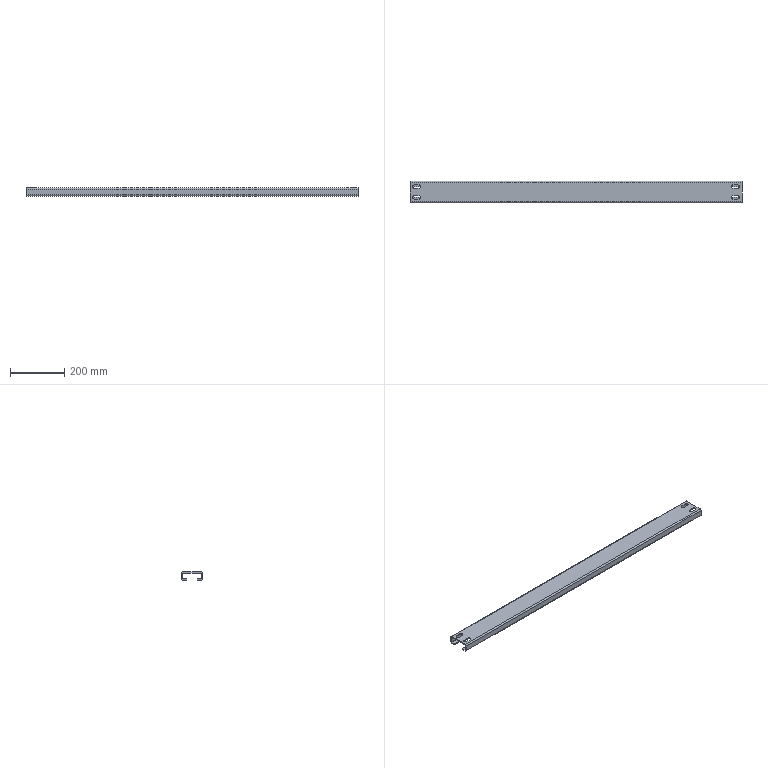Part | SolidWorks | features EdgeFlange 2, ICE 2, FlatPattern 1, SMBaseFlange 1, SheetMetal 1 | 1 solid | 58 faces | box 1228 x 80 x 30 mm | volume 774609 mm3 | plane 38 | cylinder 20 | commonest cylinder face diameters 13 x12 2 x4 10 x4